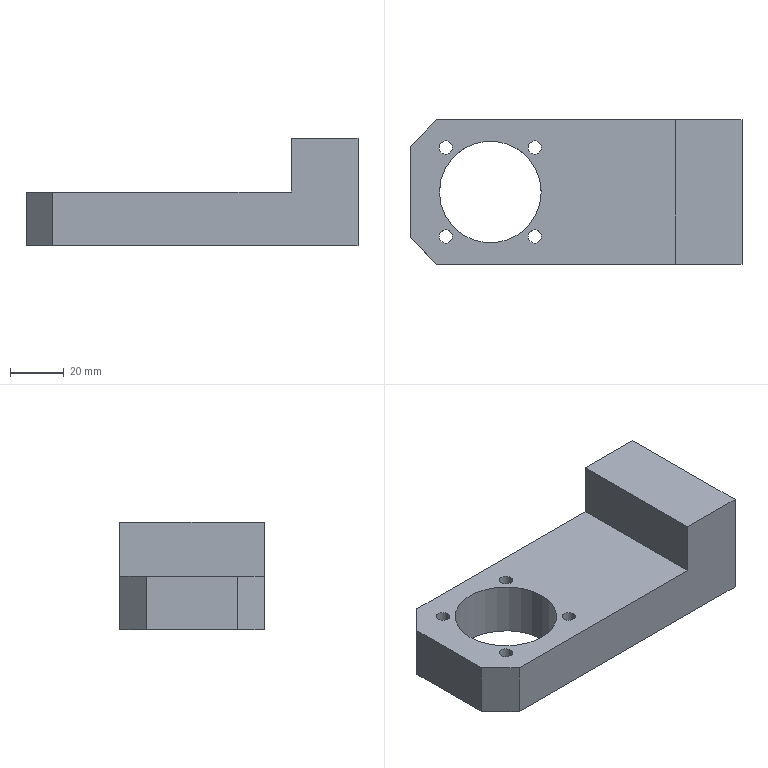Part | SolidWorks | features HoleWzd 2, ICE 2, Chamfer 1, CirPattern 1, Extrusion 1 | 1 solid | 44 faces | box 124 x 54 x 40 mm | volume 132841 mm3 | cylinder 22 | cone 12 | plane 10 | commonest cylinder face diameters 5 x20 38 x2
STEP:
#1=CARTESIAN_POINT('',(109.,47.,37.5));
#2=VERTEX_POINT('',#1);
#3=CARTESIAN_POINT('',(109.,47.,32.5));
#4=VERTEX_POINT('',#3);
#5=CARTESIAN_POINT('',(109.,47.,35.));
#6=DIRECTION('',(1.,0.,0.));
#7=DIRECTION('',(0.,0.,-1.));
#8=AXIS2_PLACEMENT_3D('',#5,#6,#7);
#9=CIRCLE('',#8,2.5);
#10=EDGE_CURVE('',#2,#4,#9,.T.);
#11=ORIENTED_EDGE('',*,*,#10,.F.);
#12=CARTESIAN_POINT('',(124.,47.,37.5));
#13=VERTEX_POINT('',#12);
#14=CARTESIAN_POINT('',(124.,47.,37.5));
#15=DIRECTION('',(1.,0.,0.));
#16=VECTOR('',#15,1000.);
#17=LINE('',#14,#16);
#18=EDGE_CURVE('',#2,#13,#17,.T.);
#19=ORIENTED_EDGE('',*,*,#18,.T.);
#20=CARTESIAN_POINT('',(124.,47.,32.5));
#21=VERTEX_POINT('',#20);
#22=CARTESIAN_POINT('',(124.,47.,35.));
#23=DIRECTION('',(1.,0.,0.));
#24=DIRECTION('',(0.,0.,-1.));
#25=AXIS2_PLACEMENT_3D('',#22,#23,#24);
#26=CIRCLE('',#25,2.5);
#27=EDGE_CURVE('',#13,#21,#26,.T.);
#28=ORIENTED_EDGE('',*,*,#27,.T.);
#29=CARTESIAN_POINT('',(124.,47.,32.5));
#30=DIRECTION('',(1.,0.,0.));
#31=VECTOR('',#30,1000.);
#32=LINE('',#29,#31);
#33=EDGE_CURVE('',#4,#21,#32,.T.);
#34=ORIENTED_EDGE('',*,*,#33,.F.);
#35=EDGE_LOOP('',(#11,#19,#28,#34));
#36=FACE_OUTER_BOUND('',#35,.T.);
#37=CARTESIAN_POINT('',(124.,47.,35.));
#38=DIRECTION('',(1.,0.,0.));
#39=DIRECTION('',(0.,0.,-1.));
#40=AXIS2_PLACEMENT_3D('',#37,#38,#39);
#41=CYLINDRICAL_SURFACE('',#40,2.5);
#42=ADVANCED_FACE('',(#36),#41,.F.);
#43=CARTESIAN_POINT('',(107.498,47.,35.));
#44=VERTEX_POINT('',#43);
#45=CARTESIAN_POINT('',(109.,47.,32.5));
#46=DIRECTION('',(0.515,0.,-0.8572));
#47=VECTOR('',#46,1000.);
#48=LINE('',#45,#47);
#49=EDGE_CURVE('',#44,#4,#48,.T.);
#50=ORIENTED_EDGE('',*,*,#49,.F.);
#51=CARTESIAN_POINT('',(109.,47.,37.5));
#52=DIRECTION('',(0.515,0.,0.8572));
#53=VECTOR('',#52,1000.);
#54=LINE('',#51,#53);
#55=EDGE_CURVE('',#44,#2,#54,.T.);
#56=ORIENTED_EDGE('',*,*,#55,.T.);
#57=ORIENTED_EDGE('',*,*,#10,.T.);
#58=EDGE_LOOP('',(#50,#56,#57));
#59=FACE_OUTER_BOUND('',#58,.T.);
#60=CARTESIAN_POINT('',(109.,47.,35.));
#61=DIRECTION('',(1.,0.,0.));
#62=DIRECTION('',(0.,0.,-1.));
#63=AXIS2_PLACEMENT_3D('',#60,#61,#62);
#64=CONICAL_SURFACE('',#63,2.5,1.03);
#65=ADVANCED_FACE('',(#59),#64,.F.);
#66=CARTESIAN_POINT('',(109.,47.,7.5));
#67=VERTEX_POINT('',#66);
#68=CARTESIAN_POINT('',(109.,47.,2.5));
#69=VERTEX_POINT('',#68);
#70=CARTESIAN_POINT('',(109.,47.,5.));
#71=DIRECTION('',(1.,0.,0.));
#72=DIRECTION('',(0.,0.,-1.));
#73=AXIS2_PLACEMENT_3D('',#70,#71,#72);
#74=CIRCLE('',#73,2.5);
#75=EDGE_CURVE('',#67,#69,#74,.T.);
#76=ORIENTED_EDGE('',*,*,#75,.F.);
#77=CARTESIAN_POINT('',(124.,47.,7.5));
#78=VERTEX_POINT('',#77);
#79=CARTESIAN_POINT('',(124.,47.,7.5));
#80=DIRECTION('',(1.,0.,0.));
#81=VECTOR('',#80,1000.);
#82=LINE('',#79,#81);
#83=EDGE_CURVE('',#67,#78,#82,.T.);
#84=ORIENTED_EDGE('',*,*,#83,.T.);
#85=CARTESIAN_POINT('',(124.,47.,2.5));
#86=VERTEX_POINT('',#85);
#87=CARTESIAN_POINT('',(124.,47.,5.));
#88=DIRECTION('',(1.,0.,0.));
#89=DIRECTION('',(0.,0.,-1.));
#90=AXIS2_PLACEMENT_3D('',#87,#88,#89);
#91=CIRCLE('',#90,2.5);
#92=EDGE_CURVE('',#78,#86,#91,.T.);
#93=ORIENTED_EDGE('',*,*,#92,.T.);
#94=CARTESIAN_POINT('',(124.,47.,2.5));
#95=DIRECTION('',(1.,0.,0.));
#96=VECTOR('',#95,1000.);
#97=LINE('',#94,#96);
#98=EDGE_CURVE('',#69,#86,#97,.T.);
#99=ORIENTED_EDGE('',*,*,#98,.F.);
#100=EDGE_LOOP('',(#76,#84,#93,#99));
#101=FACE_OUTER_BOUND('',#100,.T.);
#102=CARTESIAN_POINT('',(124.,47.,5.));
#103=DIRECTION('',(1.,0.,0.));
#104=DIRECTION('',(0.,0.,-1.));
#105=AXIS2_PLACEMENT_3D('',#102,#103,#104);
#106=CYLINDRICAL_SURFACE('',#105,2.5);
#107=ADVANCED_FACE('',(#101),#106,.F.);
#108=CARTESIAN_POINT('',(107.498,47.,5.));
#109=VERTEX_POINT('',#108);
#110=CARTESIAN_POINT('',(109.,47.,2.5));
#111=DIRECTION('',(0.515,0.,-0.8572));
#112=VECTOR('',#111,1000.);
#113=LINE('',#110,#112);
#114=EDGE_CURVE('',#109,#69,#113,.T.);
#115=ORIENTED_EDGE('',*,*,#114,.F.);
#116=CARTESIAN_POINT('',(109.,47.,7.5));
#117=DIRECTION('',(0.515,0.,0.8572));
#118=VECTOR('',#117,1000.);
#119=LINE('',#116,#118);
#120=EDGE_CURVE('',#109,#67,#119,.T.);
#121=ORIENTED_EDGE('',*,*,#120,.T.);
#122=ORIENTED_EDGE('',*,*,#75,.T.);
#123=EDGE_LOOP('',(#115,#121,#122));
#124=FACE_OUTER_BOUND('',#123,.T.);
#125=CARTESIAN_POINT('',(109.,47.,5.));
#126=DIRECTION('',(1.,0.,0.));
#127=DIRECTION('',(0.,0.,-1.));
#128=AXIS2_PLACEMENT_3D('',#125,#126,#127);
#129=CONICAL_SURFACE('',#128,2.5,1.03);
#130=ADVANCED_FACE('',(#124),#129,.F.);
#131=CARTESIAN_POINT('',(109.,7.,37.5));
#132=VERTEX_POINT('',#131);
#133=CARTESIAN_POINT('',(109.,7.,32.5));
#134=VERTEX_POINT('',#133);
#135=CARTESIAN_POINT('',(109.,7.,35.));
#136=DIRECTION('',(1.,0.,0.));
#137=DIRECTION('',(0.,0.,-1.));
#138=AXIS2_PLACEMENT_3D('',#135,#136,#137);
#139=CIRCLE('',#138,2.5);
#140=EDGE_CURVE('',#132,#134,#139,.T.);
#141=ORIENTED_EDGE('',*,*,#140,.F.);
#142=CARTESIAN_POINT('',(124.,7.,37.5));
#143=VERTEX_POINT('',#142);
#144=CARTESIAN_POINT('',(124.,7.,37.5));
#145=DIRECTION('',(1.,0.,0.));
#146=VECTOR('',#145,1000.);
#147=LINE('',#144,#146);
#148=EDGE_CURVE('',#132,#143,#147,.T.);
#149=ORIENTED_EDGE('',*,*,#148,.T.);
#150=CARTESIAN_POINT('',(124.,7.,32.5));
#151=VERTEX_POINT('',#150);
#152=CARTESIAN_POINT('',(124.,7.,35.));
#153=DIRECTION('',(1.,0.,0.));
#154=DIRECTION('',(0.,0.,-1.));
#155=AXIS2_PLACEMENT_3D('',#152,#153,#154);
#156=CIRCLE('',#155,2.5);
#157=EDGE_CURVE('',#143,#151,#156,.T.);
#158=ORIENTED_EDGE('',*,*,#157,.T.);
#159=CARTESIAN_POINT('',(124.,7.,32.5));
#160=DIRECTION('',(1.,0.,0.));
#161=VECTOR('',#160,1000.);
#162=LINE('',#159,#161);
#163=EDGE_CURVE('',#134,#151,#162,.T.);
#164=ORIENTED_EDGE('',*,*,#163,.F.);
#165=EDGE_LOOP('',(#141,#149,#158,#164));
#166=FACE_OUTER_BOUND('',#165,.T.);
#167=CARTESIAN_POINT('',(124.,7.,35.));
#168=DIRECTION('',(1.,0.,0.));
#169=DIRECTION('',(0.,0.,-1.));
#170=AXIS2_PLACEMENT_3D('',#167,#168,#169);
#171=CYLINDRICAL_SURFACE('',#170,2.5);
#172=ADVANCED_FACE('',(#166),#171,.F.);
#173=CARTESIAN_POINT('',(107.498,7.,35.));
#174=VERTEX_POINT('',#173);
#175=CARTESIAN_POINT('',(109.,7.,32.5));
#176=DIRECTION('',(0.515,0.,-0.8572));
#177=VECTOR('',#176,1000.);
#178=LINE('',#175,#177);
#179=EDGE_CURVE('',#174,#134,#178,.T.);
#180=ORIENTED_EDGE('',*,*,#179,.F.);
#181=CARTESIAN_POINT('',(109.,7.,37.5));
#182=DIRECTION('',(0.515,0.,0.8572));
#183=VECTOR('',#182,1000.);
#184=LINE('',#181,#183);
#185=EDGE_CURVE('',#174,#132,#184,.T.);
#186=ORIENTED_EDGE('',*,*,#185,.T.);
#187=ORIENTED_EDGE('',*,*,#140,.T.);
#188=EDGE_LOOP('',(#180,#186,#187));
#189=FACE_OUTER_BOUND('',#188,.T.);
#190=CARTESIAN_POINT('',(109.,7.,35.));
#191=DIRECTION('',(1.,0.,0.));
#192=DIRECTION('',(0.,0.,-1.));
#193=AXIS2_PLACEMENT_3D('',#190,#191,#192);
#194=CONICAL_SURFACE('',#193,2.5,1.03);
#195=ADVANCED_FACE('',(#189),#194,.F.);
#196=CARTESIAN_POINT('',(109.,7.,7.5));
#197=VERTEX_POINT('',#196);
#198=CARTESIAN_POINT('',(109.,7.,2.5));
#199=VERTEX_POINT('',#198);
#200=CARTESIAN_POINT('',(109.,7.,5.));
#201=DIRECTION('',(1.,0.,0.));
#202=DIRECTION('',(0.,0.,-1.));
#203=AXIS2_PLACEMENT_3D('',#200,#201,#202);
#204=CIRCLE('',#203,2.5);
#205=EDGE_CURVE('',#197,#199,#204,.T.);
#206=ORIENTED_EDGE('',*,*,#205,.F.);
#207=CARTESIAN_POINT('',(124.,7.,7.5));
#208=VERTEX_POINT('',#207);
#209=CARTESIAN_POINT('',(124.,7.,7.5));
#210=DIRECTION('',(1.,0.,0.));
#211=VECTOR('',#210,1000.);
#212=LINE('',#209,#211);
#213=EDGE_CURVE('',#197,#208,#212,.T.);
#214=ORIENTED_EDGE('',*,*,#213,.T.);
#215=CARTESIAN_POINT('',(124.,7.,2.5));
#216=VERTEX_POINT('',#215);
#217=CARTESIAN_POINT('',(124.,7.,5.));
#218=DIRECTION('',(1.,0.,0.));
#219=DIRECTION('',(0.,0.,-1.));
#220=AXIS2_PLACEMENT_3D('',#217,#218,#219);
#221=CIRCLE('',#220,2.5);
#222=EDGE_CURVE('',#208,#216,#221,.T.);
#223=ORIENTED_EDGE('',*,*,#222,.T.);
#224=CARTESIAN_POINT('',(124.,7.,2.5));
#225=DIRECTION('',(1.,0.,0.));
#226=VECTOR('',#225,1000.);
#227=LINE('',#224,#226);
#228=EDGE_CURVE('',#199,#216,#227,.T.);
#229=ORIENTED_EDGE('',*,*,#228,.F.);
#230=EDGE_LOOP('',(#206,#214,#223,#229));
#231=FACE_OUTER_BOUND('',#230,.T.);
#232=CARTESIAN_POINT('',(124.,7.,5.));
#233=DIRECTION('',(1.,0.,0.));
#234=DIRECTION('',(0.,0.,-1.));
#235=AXIS2_PLACEMENT_3D('',#232,#233,#234);
#236=CYLINDRICAL_SURFACE('',#235,2.5);
#237=ADVANCED_FACE('',(#231),#236,.F.);
#238=CARTESIAN_POINT('',(107.498,7.,5.));
#239=VERTEX_POINT('',#238);
#240=CARTESIAN_POINT('',(109.,7.,2.5));
#241=DIRECTION('',(0.515,0.,-0.8572));
#242=VECTOR('',#241,1000.);
#243=LINE('',#240,#242);
#244=EDGE_CURVE('',#239,#199,#243,.T.);
#245=ORIENTED_EDGE('',*,*,#244,.F.);
#246=CARTESIAN_POINT('',(109.,7.,7.5));
#247=DIRECTION('',(0.515,0.,0.8572));
#248=VECTOR('',#247,1000.);
#249=LINE('',#246,#248);
#250=EDGE_CURVE('',#239,#197,#249,.T.);
#251=ORIENTED_EDGE('',*,*,#250,.T.);
#252=ORIENTED_EDGE('',*,*,#205,.T.);
#253=EDGE_LOOP('',(#245,#251,#252));
#254=FACE_OUTER_BOUND('',#253,.T.);
#255=CARTESIAN_POINT('',(109.,7.,5.));
#256=DIRECTION('',(1.,0.,0.));
#257=DIRECTION('',(0.,0.,-1.));
#258=AXIS2_PLACEMENT_3D('',#255,#256,#257);
#259=CONICAL_SURFACE('',#258,2.5,1.03);
#260=ADVANCED_FACE('',(#254),#259,.F.);
#261=CARTESIAN_POINT('',(109.,27.,37.5));
#262=VERTEX_POINT('',#261);
#263=CARTESIAN_POINT('',(109.,27.,32.5));
#264=VERTEX_POINT('',#263);
#265=CARTESIAN_POINT('',(109.,27.,35.));
#266=DIRECTION('',(1.,0.,0.));
#267=DIRECTION('',(0.,0.,-1.));
#268=AXIS2_PLACEMENT_3D('',#265,#266,#267);
#269=CIRCLE('',#268,2.5);
#270=EDGE_CURVE('',#262,#264,#269,.T.);
#271=ORIENTED_EDGE('',*,*,#270,.F.);
#272=CARTESIAN_POINT('',(124.,27.,37.5));
#273=VERTEX_POINT('',#272);
#274=CARTESIAN_POINT('',(124.,27.,37.5));
#275=DIRECTION('',(1.,0.,0.));
#276=VECTOR('',#275,1000.);
#277=LINE('',#274,#276);
#278=EDGE_CURVE('',#262,#273,#277,.T.);
#279=ORIENTED_EDGE('',*,*,#278,.T.);
#280=CARTESIAN_POINT('',(124.,27.,32.5));
#281=VERTEX_POINT('',#280);
#282=CARTESIAN_POINT('',(124.,27.,35.));
#283=DIRECTION('',(1.,0.,0.));
#284=DIRECTION('',(0.,0.,-1.));
#285=AXIS2_PLACEMENT_3D('',#282,#283,#284);
#286=CIRCLE('',#285,2.5);
#287=EDGE_CURVE('',#273,#281,#286,.T.);
#288=ORIENTED_EDGE('',*,*,#287,.T.);
#289=CARTESIAN_POINT('',(124.,27.,32.5));
#290=DIRECTION('',(1.,0.,0.));
#291=VECTOR('',#290,1000.);
#292=LINE('',#289,#291);
#293=EDGE_CURVE('',#264,#281,#292,.T.);
#294=ORIENTED_EDGE('',*,*,#293,.F.);
#295=EDGE_LOOP('',(#271,#279,#288,#294));
#296=FACE_OUTER_BOUND('',#295,.T.);
#297=CARTESIAN_POINT('',(124.,27.,35.));
#298=DIRECTION('',(1.,0.,0.));
#299=DIRECTION('',(0.,0.,-1.));
#300=AXIS2_PLACEMENT_3D('',#297,#298,#299);
#301=CYLINDRICAL_SURFACE('',#300,2.5);
#302=ADVANCED_FACE('',(#296),#301,.F.);
#303=CARTESIAN_POINT('',(107.498,27.,35.));
#304=VERTEX_POINT('',#303);
#305=CARTESIAN_POINT('',(109.,27.,32.5));
#306=DIRECTION('',(0.515,0.,-0.8572));
#307=VECTOR('',#306,1000.);
#308=LINE('',#305,#307);
#309=EDGE_CURVE('',#304,#264,#308,.T.);
#310=ORIENTED_EDGE('',*,*,#309,.F.);
#311=CARTESIAN_POINT('',(109.,27.,37.5));
#312=DIRECTION('',(0.515,0.,0.8572));
#313=VECTOR('',#312,1000.);
#314=LINE('',#311,#313);
#315=EDGE_CURVE('',#304,#262,#314,.T.);
#316=ORIENTED_EDGE('',*,*,#315,.T.);
#317=ORIENTED_EDGE('',*,*,#270,.T.);
#318=EDGE_LOOP('',(#310,#316,#317));
#319=FACE_OUTER_BOUND('',#318,.T.);
#320=CARTESIAN_POINT('',(109.,27.,35.));
#321=DIRECTION('',(1.,0.,0.));
#322=DIRECTION('',(0.,0.,-1.));
#323=AXIS2_PLACEMENT_3D('',#320,#321,#322);
#324=CONICAL_SURFACE('',#323,2.5,1.03);
#325=ADVANCED_FACE('',(#319),#324,.F.);
#326=CARTESIAN_POINT('',(109.,27.,7.5));
#327=VERTEX_POINT('',#326);
#328=CARTESIAN_POINT('',(109.,27.,2.5));
#329=VERTEX_POINT('',#328);
#330=CARTESIAN_POINT('',(109.,27.,5.));
#331=DIRECTION('',(1.,0.,0.));
#332=DIRECTION('',(0.,0.,-1.));
#333=AXIS2_PLACEMENT_3D('',#330,#331,#332);
#334=CIRCLE('',#333,2.5);
#335=EDGE_CURVE('',#327,#329,#334,.T.);
#336=ORIENTED_EDGE('',*,*,#335,.F.);
#337=CARTESIAN_POINT('',(124.,27.,7.5));
#338=VERTEX_POINT('',#337);
#339=CARTESIAN_POINT('',(124.,27.,7.5));
#340=DIRECTION('',(1.,0.,0.));
#341=VECTOR('',#340,1000.);
#342=LINE('',#339,#341);
#343=EDGE_CURVE('',#327,#338,#342,.T.);
#344=ORIENTED_EDGE('',*,*,#343,.T.);
#345=CARTESIAN_POINT('',(124.,27.,2.5));
#346=VERTEX_POINT('',#345);
#347=CARTESIAN_POINT('',(124.,27.,5.));
#348=DIRECTION('',(1.,0.,0.));
#349=DIRECTION('',(0.,0.,-1.));
#350=AXIS2_PLACEMENT_3D('',#347,#348,#349);
#351=CIRCLE('',#350,2.5);
#352=EDGE_CURVE('',#338,#346,#351,.T.);
#353=ORIENTED_EDGE('',*,*,#352,.T.);
#354=CARTESIAN_POINT('',(124.,27.,2.5));
#355=DIRECTION('',(1.,0.,0.));
#356=VECTOR('',#355,1000.);
#357=LINE('',#354,#356);
#358=EDGE_CURVE('',#329,#346,#357,.T.);
#359=ORIENTED_EDGE('',*,*,#358,.F.);
#360=EDGE_LOOP('',(#336,#344,#353,#359));
#361=FACE_OUTER_BOUND('',#360,.T.);
#362=CARTESIAN_POINT('',(124.,27.,5.));
#363=DIRECTION('',(1.,0.,0.));
#364=DIRECTION('',(0.,0.,-1.));
#365=AXIS2_PLACEMENT_3D('',#362,#363,#364);
#366=CYLINDRICAL_SURFACE('',#365,2.5);
#367=ADVANCED_FACE('',(#361),#366,.F.);
#368=CARTESIAN_POINT('',(107.498,27.,5.));
#369=VERTEX_POINT('',#368);
#370=CARTESIAN_POINT('',(109.,27.,2.5));
#371=DIRECTION('',(0.515,0.,-0.8572));
#372=VECTOR('',#371,1000.);
#373=LINE('',#370,#372);
#374=EDGE_CURVE('',#369,#329,#373,.T.);
#375=ORIENTED_EDGE('',*,*,#374,.F.);
#376=CARTESIAN_POINT('',(109.,27.,7.5));
#377=DIRECTION('',(0.515,0.,0.8572));
#378=VECTOR('',#377,1000.);
#379=LINE('',#376,#378);
#380=EDGE_CURVE('',#369,#327,#379,.T.);
#381=ORIENTED_EDGE('',*,*,#380,.T.);
#382=ORIENTED_EDGE('',*,*,#335,.T.);
#383=EDGE_LOOP('',(#375,#381,#382));
#384=FACE_OUTER_BOUND('',#383,.T.);
#385=CARTESIAN_POINT('',(109.,27.,5.));
#386=DIRECTION('',(1.,0.,0.));
#387=DIRECTION('',(0.,0.,-1.));
#388=AXIS2_PLACEMENT_3D('',#385,#386,#387);
#389=CONICAL_SURFACE('',#388,2.5,1.03);
#390=ADVANCED_FACE('',(#384),#389,.F.);
#391=CARTESIAN_POINT('',(44.117,10.383,0.));
#392=VERTEX_POINT('',#391);
#393=CARTESIAN_POINT('',(49.117,10.383,0.));
#394=VERTEX_POINT('',#393);
#395=CARTESIAN_POINT('',(46.617,10.383,0.));
#396=DIRECTION('',(0.,0.,1.));
#397=DIRECTION('',(1.,0.,0.));
#398=AXIS2_PLACEMENT_3D('',#395,#396,#397);
#399=CIRCLE('',#398,2.5);
#400=EDGE_CURVE('',#392,#394,#399,.T.);
#401=ORIENTED_EDGE('',*,*,#400,.F.);
#402=CARTESIAN_POINT('',(44.117,10.383,20.));
#403=VERTEX_POINT('',#402);
#404=CARTESIAN_POINT('',(44.117,10.383,20.));
#405=DIRECTION('',(0.,0.,1.));
#406=VECTOR('',#405,1000.);
#407=LINE('',#404,#406);
#408=EDGE_CURVE('',#392,#403,#407,.T.);
#409=ORIENTED_EDGE('',*,*,#408,.T.);
#410=CARTESIAN_POINT('',(49.117,10.383,20.));
#411=VERTEX_POINT('',#410);
#412=CARTESIAN_POINT('',(46.617,10.383,20.));
#413=DIRECTION('',(0.,0.,1.));
#414=DIRECTION('',(1.,0.,0.));
#415=AXIS2_PLACEMENT_3D('',#412,#413,#414);
#416=CIRCLE('',#415,2.5);
#417=EDGE_CURVE('',#403,#411,#416,.T.);
#418=ORIENTED_EDGE('',*,*,#417,.T.);
#419=CARTESIAN_POINT('',(49.117,10.383,20.));
#420=DIRECTION('',(0.,0.,1.));
#421=VECTOR('',#420,1000.);
#422=LINE('',#419,#421);
#423=EDGE_CURVE('',#394,#411,#422,.T.);
#424=ORIENTED_EDGE('',*,*,#423,.F.);
#425=EDGE_LOOP('',(#401,#409,#418,#424));
#426=FACE_OUTER_BOUND('',#425,.T.);
#427=CARTESIAN_POINT('',(46.617,10.383,20.));
#428=DIRECTION('',(0.,0.,1.));
#429=DIRECTION('',(1.,0.,0.));
#430=AXIS2_PLACEMENT_3D('',#427,#428,#429);
#431=CYLINDRICAL_SURFACE('',#430,2.5);
#432=ADVANCED_FACE('',(#426),#431,.F.);
#433=CARTESIAN_POINT('',(10.883,10.383,0.));
#434=VERTEX_POINT('',#433);
#435=CARTESIAN_POINT('',(15.883,10.383,0.));
#436=VERTEX_POINT('',#435);
#437=CARTESIAN_POINT('',(13.383,10.383,0.));
#438=DIRECTION('',(0.,0.,1.));
#439=DIRECTION('',(1.,0.,0.));
#440=AXIS2_PLACEMENT_3D('',#437,#438,#439);
#441=CIRCLE('',#440,2.5);
#442=EDGE_CURVE('',#434,#436,#441,.T.);
#443=ORIENTED_EDGE('',*,*,#442,.F.);
#444=CARTESIAN_POINT('',(10.883,10.383,20.));
#445=VERTEX_POINT('',#444);
#446=CARTESIAN_POINT('',(10.883,10.383,20.));
#447=DIRECTION('',(0.,0.,1.));
#448=VECTOR('',#447,1000.);
#449=LINE('',#446,#448);
#450=EDGE_CURVE('',#434,#445,#449,.T.);
#451=ORIENTED_EDGE('',*,*,#450,.T.);
#452=CARTESIAN_POINT('',(15.883,10.383,20.));
#453=VERTEX_POINT('',#452);
#454=CARTESIAN_POINT('',(13.383,10.383,20.));
#455=DIRECTION('',(0.,0.,1.));
#456=DIRECTION('',(1.,0.,0.));
#457=AXIS2_PLACEMENT_3D('',#454,#455,#456);
#458=CIRCLE('',#457,2.5);
#459=EDGE_CURVE('',#445,#453,#458,.T.);
#460=ORIENTED_EDGE('',*,*,#459,.T.);
#461=CARTESIAN_POINT('',(15.883,10.383,20.));
#462=DIRECTION('',(0.,0.,1.));
#463=VECTOR('',#462,1000.);
#464=LINE('',#461,#463);
#465=EDGE_CURVE('',#436,#453,#464,.T.);
#466=ORIENTED_EDGE('',*,*,#465,.F.);
#467=EDGE_LOOP('',(#443,#451,#460,#466));
#468=FACE_OUTER_BOUND('',#467,.T.);
#469=CARTESIAN_POINT('',(13.383,10.383,20.));
#470=DIRECTION('',(0.,0.,1.));
#471=DIRECTION('',(1.,0.,0.));
#472=AXIS2_PLACEMENT_3D('',#469,#470,#471);
#473=CYLINDRICAL_SURFACE('',#472,2.5);
#474=ADVANCED_FACE('',(#468),#473,.F.);
#475=CARTESIAN_POINT('',(10.883,43.617,0.));
#476=VERTEX_POINT('',#475);
#477=CARTESIAN_POINT('',(15.883,43.617,0.));
#478=VERTEX_POINT('',#477);
#479=CARTESIAN_POINT('',(13.383,43.617,0.));
#480=DIRECTION('',(0.,0.,1.));
#481=DIRECTION('',(1.,0.,0.));
#482=AXIS2_PLACEMENT_3D('',#479,#480,#481);
#483=CIRCLE('',#482,2.5);
#484=EDGE_CURVE('',#476,#478,#483,.T.);
#485=ORIENTED_EDGE('',*,*,#484,.F.);
#486=CARTESIAN_POINT('',(10.883,43.617,20.));
#487=VERTEX_POINT('',#486);
#488=CARTESIAN_POINT('',(10.883,43.617,20.));
#489=DIRECTION('',(0.,0.,1.));
#490=VECTOR('',#489,1000.);
#491=LINE('',#488,#490);
#492=EDGE_CURVE('',#476,#487,#491,.T.);
#493=ORIENTED_EDGE('',*,*,#492,.T.);
#494=CARTESIAN_POINT('',(15.883,43.617,20.));
#495=VERTEX_POINT('',#494);
#496=CARTESIAN_POINT('',(13.383,43.617,20.));
#497=DIRECTION('',(0.,0.,1.));
#498=DIRECTION('',(1.,0.,0.));
#499=AXIS2_PLACEMENT_3D('',#496,#497,#498);
#500=CIRCLE('',#499,2.5);
#501=EDGE_CURVE('',#487,#495,#500,.T.);
#502=ORIENTED_EDGE('',*,*,#501,.T.);
#503=CARTESIAN_POINT('',(15.883,43.617,20.));
#504=DIRECTION('',(0.,0.,1.));
#505=VECTOR('',#504,1000.);
#506=LINE('',#503,#505);
#507=EDGE_CURVE('',#478,#495,#506,.T.);
#508=ORIENTED_EDGE('',*,*,#507,.F.);
#509=EDGE_LOOP('',(#485,#493,#502,#508));
#510=FACE_OUTER_BOUND('',#509,.T.);
#511=CARTESIAN_POINT('',(13.383,43.617,20.));
#512=DIRECTION('',(0.,0.,1.));
#513=DIRECTION('',(1.,0.,0.));
#514=AXIS2_PLACEMENT_3D('',#511,#512,#513);
#515=CYLINDRICAL_SURFACE('',#514,2.5);
#516=ADVANCED_FACE('',(#510),#515,.F.);
#517=CARTESIAN_POINT('',(44.117,43.617,0.));
#518=VERTEX_POINT('',#517);
#519=CARTESIAN_POINT('',(49.117,43.617,0.));
#520=VERTEX_POINT('',#519);
#521=CARTESIAN_POINT('',(46.617,43.617,0.));
#522=DIRECTION('',(0.,0.,1.));
#523=DIRECTION('',(1.,0.,0.));
#524=AXIS2_PLACEMENT_3D('',#521,#522,#523);
#525=CIRCLE('',#524,2.5);
#526=EDGE_CURVE('',#518,#520,#525,.T.);
#527=ORIENTED_EDGE('',*,*,#526,.F.);
#528=CARTESIAN_POINT('',(44.117,43.617,20.));
#529=VERTEX_POINT('',#528);
#530=CARTESIAN_POINT('',(44.117,43.617,20.));
#531=DIRECTION('',(0.,0.,1.));
#532=VECTOR('',#531,1000.);
#533=LINE('',#530,#532);
#534=EDGE_CURVE('',#518,#529,#533,.T.);
#535=ORIENTED_EDGE('',*,*,#534,.T.);
#536=CARTESIAN_POINT('',(49.117,43.617,20.));
#537=VERTEX_POINT('',#536);
#538=CARTESIAN_POINT('',(46.617,43.617,20.));
#539=DIRECTION('',(0.,0.,1.));
#540=DIRECTION('',(1.,0.,0.));
#541=AXIS2_PLACEMENT_3D('',#538,#539,#540);
#542=CIRCLE('',#541,2.5);
#543=EDGE_CURVE('',#529,#537,#542,.T.);
#544=ORIENTED_EDGE('',*,*,#543,.T.);
#545=CARTESIAN_POINT('',(49.117,43.617,20.));
#546=DIRECTION('',(0.,0.,1.));
#547=VECTOR('',#546,1000.);
#548=LINE('',#545,#547);
#549=EDGE_CURVE('',#520,#537,#548,.T.);
#550=ORIENTED_EDGE('',*,*,#549,.F.);
#551=EDGE_LOOP('',(#527,#535,#544,#550));
#552=FACE_OUTER_BOUND('',#551,.T.);
#553=CARTESIAN_POINT('',(46.617,43.617,20.));
#554=DIRECTION('',(0.,0.,1.));
#555=DIRECTION('',(1.,0.,0.));
#556=AXIS2_PLACEMENT_3D('',#553,#554,#555);
#557=CYLINDRICAL_SURFACE('',#556,2.5);
#558=ADVANCED_FACE('',(#552),#557,.F.);
#559=CARTESIAN_POINT('',(11.,27.,0.));
#560=VERTEX_POINT('',#559);
#561=CARTESIAN_POINT('',(49.,27.,0.));
#562=VERTEX_POINT('',#561);
#563=CARTESIAN_POINT('',(30.,27.,0.));
#564=DIRECTION('',(0.,0.,1.));
#565=DIRECTION('',(1.,0.,0.));
#566=AXIS2_PLACEMENT_3D('',#563,#564,#565);
#567=CIRCLE('',#566,19.);
#568=EDGE_CURVE('',#560,#562,#567,.T.);
#569=ORIENTED_EDGE('',*,*,#568,.F.);
#570=CARTESIAN_POINT('',(11.,27.,20.));
#571=VERTEX_POINT('',#570);
#572=CARTESIAN_POINT('',(11.,27.,0.));
#573=DIRECTION('',(0.,0.,1.));
#574=VECTOR('',#573,1000.);
#575=LINE('',#572,#574);
#576=EDGE_CURVE('',#560,#571,#575,.T.);
#577=ORIENTED_EDGE('',*,*,#576,.T.);
#578=CARTESIAN_POINT('',(49.,27.,20.));
#579=VERTEX_POINT('',#578);
#580=CARTESIAN_POINT('',(30.,27.,20.));
#581=DIRECTION('',(0.,0.,1.));
#582=DIRECTION('',(1.,0.,0.));
#583=AXIS2_PLACEMENT_3D('',#580,#581,#582);
#584=CIRCLE('',#583,19.);
#585=EDGE_CURVE('',#571,#579,#584,.T.);
#586=ORIENTED_EDGE('',*,*,#585,.T.);
#587=CARTESIAN_POINT('',(49.,27.,0.));
#588=DIRECTION('',(0.,0.,1.));
#589=VECTOR('',#588,1000.);
#590=LINE('',#587,#589);
#591=EDGE_CURVE('',#562,#579,#590,.T.);
#592=ORIENTED_EDGE('',*,*,#591,.F.);
#593=EDGE_LOOP('',(#569,#577,#586,#592));
#594=FACE_OUTER_BOUND('',#593,.T.);
#595=CARTESIAN_POINT('',(30.,27.,0.));
#596=DIRECTION('',(0.,0.,1.));
#597=DIRECTION('',(1.,0.,0.));
#598=AXIS2_PLACEMENT_3D('',#595,#596,#597);
#599=CYLINDRICAL_SURFACE('',#598,19.);
#600=ADVANCED_FACE('',(#594),#599,.F.);
#601=CARTESIAN_POINT('',(30.,27.,20.));
#602=DIRECTION('',(0.,0.,1.));
#603=DIRECTION('',(1.,0.,0.));
#604=AXIS2_PLACEMENT_3D('',#601,#602,#603);
#605=CIRCLE('',#604,19.);
#606=EDGE_CURVE('',#579,#571,#605,.T.);
#607=ORIENTED_EDGE('',*,*,#606,.F.);
#608=ORIENTED_EDGE('',*,*,#585,.F.);
#609=EDGE_LOOP('',(#607,#608));
#610=FACE_BOUND('',#609,.T.);
#611=CARTESIAN_POINT('',(46.617,43.617,20.));
#612=DIRECTION('',(0.,0.,1.));
#613=DIRECTION('',(1.,0.,0.));
#614=AXIS2_PLACEMENT_3D('',#611,#612,#613);
#615=CIRCLE('',#614,2.5);
#616=EDGE_CURVE('',#537,#529,#615,.T.);
#617=ORIENTED_EDGE('',*,*,#616,.F.);
#618=ORIENTED_EDGE('',*,*,#543,.F.);
#619=EDGE_LOOP('',(#617,#618));
#620=FACE_BOUND('',#619,.T.);
#621=CARTESIAN_POINT('',(13.383,43.617,20.));
#622=DIRECTION('',(0.,0.,1.));
#623=DIRECTION('',(1.,0.,0.));
#624=AXIS2_PLACEMENT_3D('',#621,#622,#623);
#625=CIRCLE('',#624,2.5);
#626=EDGE_CURVE('',#495,#487,#625,.T.);
#627=ORIENTED_EDGE('',*,*,#626,.F.);
#628=ORIENTED_EDGE('',*,*,#501,.F.);
#629=EDGE_LOOP('',(#627,#628));
#630=FACE_BOUND('',#629,.T.);
#631=CARTESIAN_POINT('',(13.383,10.383,20.));
#632=DIRECTION('',(0.,0.,1.));
#633=DIRECTION('',(1.,0.,0.));
#634=AXIS2_PLACEMENT_3D('',#631,#632,#633);
#635=CIRCLE('',#634,2.5);
#636=EDGE_CURVE('',#453,#445,#635,.T.);
#637=ORIENTED_EDGE('',*,*,#636,.F.);
#638=ORIENTED_EDGE('',*,*,#459,.F.);
#639=EDGE_LOOP('',(#637,#638));
#640=FACE_BOUND('',#639,.T.);
#641=CARTESIAN_POINT('',(46.617,10.383,20.));
#642=DIRECTION('',(0.,0.,1.));
#643=DIRECTION('',(1.,0.,0.));
#644=AXIS2_PLACEMENT_3D('',#641,#642,#643);
#645=CIRCLE('',#644,2.5);
#646=EDGE_CURVE('',#411,#403,#645,.T.);
#647=ORIENTED_EDGE('',*,*,#646,.F.);
#648=ORIENTED_EDGE('',*,*,#417,.F.);
#649=EDGE_LOOP('',(#647,#648));
#650=FACE_BOUND('',#649,.T.);
#651=CARTESIAN_POINT('',(99.,54.,20.));
#652=VERTEX_POINT('',#651);
#653=CARTESIAN_POINT('',(99.,0.,20.));
#654=VERTEX_POINT('',#653);
#655=CARTESIAN_POINT('',(99.,0.,20.));
#656=DIRECTION('',(0.,-1.,0.));
#657=VECTOR('',#656,1000.);
#658=LINE('',#655,#657);
#659=EDGE_CURVE('',#652,#654,#658,.T.);
#660=ORIENTED_EDGE('',*,*,#659,.F.);
#661=CARTESIAN_POINT('',(10.,54.,20.));
#662=VERTEX_POINT('',#661);
#663=CARTESIAN_POINT('',(0.,54.,20.));
#664=DIRECTION('',(-1.,0.,0.));
#665=VECTOR('',#664,1000.);
#666=LINE('',#663,#665);
#667=EDGE_CURVE('',#652,#662,#666,.T.);
#668=ORIENTED_EDGE('',*,*,#667,.T.);
#669=CARTESIAN_POINT('',(0.,44.,20.));
#670=VERTEX_POINT('',#669);
#671=CARTESIAN_POINT('',(0.,44.,20.));
#672=DIRECTION('',(-0.7071,-0.7071,0.));
#673=VECTOR('',#672,1000.);
#674=LINE('',#671,#673);
#675=EDGE_CURVE('',#662,#670,#674,.T.);
#676=ORIENTED_EDGE('',*,*,#675,.T.);
#677=CARTESIAN_POINT('',(0.,10.,20.));
#678=VERTEX_POINT('',#677);
#679=CARTESIAN_POINT('',(0.,0.,20.));
#680=DIRECTION('',(0.,-1.,0.));
#681=VECTOR('',#680,1000.);
#682=LINE('',#679,#681);
#683=EDGE_CURVE('',#670,#678,#682,.T.);
#684=ORIENTED_EDGE('',*,*,#683,.T.);
#685=CARTESIAN_POINT('',(10.,0.,20.));
#686=VERTEX_POINT('',#685);
#687=CARTESIAN_POINT('',(10.,0.,20.));
#688=DIRECTION('',(0.7071,-0.7071,0.));
#689=VECTOR('',#688,1000.);
#690=LINE('',#687,#689);
#691=EDGE_CURVE('',#678,#686,#690,.T.);
#692=ORIENTED_EDGE('',*,*,#691,.T.);
#693=CARTESIAN_POINT('',(0.,0.,20.));
#694=DIRECTION('',(1.,0.,0.));
#695=VECTOR('',#694,1000.);
#696=LINE('',#693,#695);
#697=EDGE_CURVE('',#686,#654,#696,.T.);
#698=ORIENTED_EDGE('',*,*,#697,.T.);
#699=EDGE_LOOP('',(#660,#668,#676,#684,#692,#698));
#700=FACE_OUTER_BOUND('',#699,.T.);
#701=CARTESIAN_POINT('',(0.,54.,20.));
#702=DIRECTION('',(0.,0.,-1.));
#703=DIRECTION('',(-1.,0.,0.));
#704=AXIS2_PLACEMENT_3D('',#701,#702,#703);
#705=PLANE('',#704);
#706=ADVANCED_FACE('',(#610,#620,#630,#640,#650,#700),#705,.F.);
#707=CARTESIAN_POINT('',(0.,44.,0.));
#708=VERTEX_POINT('',#707);
#709=CARTESIAN_POINT('',(0.,10.,0.));
#710=VERTEX_POINT('',#709);
#711=CARTESIAN_POINT('',(0.,0.,0.));
#712=DIRECTION('',(0.,-1.,0.));
#713=VECTOR('',#712,1000.);
#714=LINE('',#711,#713);
#715=EDGE_CURVE('',#708,#710,#714,.T.);
#716=ORIENTED_EDGE('',*,*,#715,.F.);
#717=CARTESIAN_POINT('',(10.,54.,0.));
#718=VERTEX_POINT('',#717);
#719=CARTESIAN_POINT('',(5.,49.,0.));
#720=DIRECTION('',(0.7071,0.7071,0.));
#721=VECTOR('',#720,1000.);
#722=LINE('',#719,#721);
#723=EDGE_CURVE('',#708,#718,#722,.T.);
#724=ORIENTED_EDGE('',*,*,#723,.T.);
#725=CARTESIAN_POINT('',(124.,54.,0.));
#726=VERTEX_POINT('',#725);
#727=CARTESIAN_POINT('',(0.,54.,0.));
#728=DIRECTION('',(-1.,0.,0.));
#729=VECTOR('',#728,1000.);
#730=LINE('',#727,#729);
#731=EDGE_CURVE('',#726,#718,#730,.T.);
#732=ORIENTED_EDGE('',*,*,#731,.F.);
#733=CARTESIAN_POINT('',(124.,0.,0.));
#734=VERTEX_POINT('',#733);
#735=CARTESIAN_POINT('',(124.,0.,0.));
#736=DIRECTION('',(0.,1.,0.));
#737=VECTOR('',#736,1000.);
#738=LINE('',#735,#737);
#739=EDGE_CURVE('',#734,#726,#738,.T.);
#740=ORIENTED_EDGE('',*,*,#739,.F.);
#741=CARTESIAN_POINT('',(10.,0.,0.));
#742=VERTEX_POINT('',#741);
#743=CARTESIAN_POINT('',(0.,0.,0.));
#744=DIRECTION('',(1.,0.,0.));
#745=VECTOR('',#744,1000.);
#746=LINE('',#743,#745);
#747=EDGE_CURVE('',#742,#734,#746,.T.);
#748=ORIENTED_EDGE('',*,*,#747,.F.);
#749=CARTESIAN_POINT('',(-22.,32.,0.));
#750=DIRECTION('',(-0.7071,0.7071,0.));
#751=VECTOR('',#750,1000.);
#752=LINE('',#749,#751);
#753=EDGE_CURVE('',#742,#710,#752,.T.);
#754=ORIENTED_EDGE('',*,*,#753,.T.);
#755=EDGE_LOOP('',(#716,#724,#732,#740,#748,#754));
#756=FACE_OUTER_BOUND('',#755,.T.);
#757=CARTESIAN_POINT('',(30.,27.,0.));
#758=DIRECTION('',(0.,0.,1.));
#759=DIRECTION('',(1.,0.,0.));
#760=AXIS2_PLACEMENT_3D('',#757,#758,#759);
#761=CIRCLE('',#760,19.);
#762=EDGE_CURVE('',#562,#560,#761,.T.);
#763=ORIENTED_EDGE('',*,*,#762,.T.);
#764=ORIENTED_EDGE('',*,*,#568,.T.);
#765=EDGE_LOOP('',(#763,#764));
#766=FACE_BOUND('',#765,.T.);
#767=CARTESIAN_POINT('',(46.617,43.617,0.));
#768=DIRECTION('',(0.,0.,1.));
#769=DIRECTION('',(1.,0.,0.));
#770=AXIS2_PLACEMENT_3D('',#767,#768,#769);
#771=CIRCLE('',#770,2.5);
#772=EDGE_CURVE('',#520,#518,#771,.T.);
#773=ORIENTED_EDGE('',*,*,#772,.T.);
#774=ORIENTED_EDGE('',*,*,#526,.T.);
#775=EDGE_LOOP('',(#773,#774));
#776=FACE_BOUND('',#775,.T.);
#777=CARTESIAN_POINT('',(13.383,43.617,0.));
#778=DIRECTION('',(0.,0.,1.));
#779=DIRECTION('',(1.,0.,0.));
#780=AXIS2_PLACEMENT_3D('',#777,#778,#779);
#781=CIRCLE('',#780,2.5);
#782=EDGE_CURVE('',#478,#476,#781,.T.);
#783=ORIENTED_EDGE('',*,*,#782,.T.);
#784=ORIENTED_EDGE('',*,*,#484,.T.);
#785=EDGE_LOOP('',(#783,#784));
#786=FACE_BOUND('',#785,.T.);
#787=CARTESIAN_POINT('',(13.383,10.383,0.));
#788=DIRECTION('',(0.,0.,1.));
#789=DIRECTION('',(1.,0.,0.));
#790=AXIS2_PLACEMENT_3D('',#787,#788,#789);
#791=CIRCLE('',#790,2.5);
#792=EDGE_CURVE('',#436,#434,#791,.T.);
#793=ORIENTED_EDGE('',*,*,#792,.T.);
#794=ORIENTED_EDGE('',*,*,#442,.T.);
#795=EDGE_LOOP('',(#793,#794));
#796=FACE_BOUND('',#795,.T.);
#797=CARTESIAN_POINT('',(46.617,10.383,0.));
#798=DIRECTION('',(0.,0.,1.));
#799=DIRECTION('',(1.,0.,0.));
#800=AXIS2_PLACEMENT_3D('',#797,#798,#799);
#801=CIRCLE('',#800,2.5);
#802=EDGE_CURVE('',#394,#392,#801,.T.);
#803=ORIENTED_EDGE('',*,*,#802,.T.);
#804=ORIENTED_EDGE('',*,*,#400,.T.);
#805=EDGE_LOOP('',(#803,#804));
#806=FACE_BOUND('',#805,.T.);
#807=CARTESIAN_POINT('',(0.,54.,0.));
#808=DIRECTION('',(0.,0.,-1.));
#809=DIRECTION('',(-1.,0.,0.));
#810=AXIS2_PLACEMENT_3D('',#807,#808,#809);
#811=PLANE('',#810);
#812=ADVANCED_FACE('',(#756,#766,#776,#786,#796,#806),#811,.T.);
#813=ORIENTED_EDGE('',*,*,#683,.F.);
#814=CARTESIAN_POINT('',(0.,44.,20.));
#815=DIRECTION('',(0.,0.,-1.));
#816=VECTOR('',#815,1000.);
#817=LINE('',#814,#816);
#818=EDGE_CURVE('',#670,#708,#817,.T.);
#819=ORIENTED_EDGE('',*,*,#818,.T.);
#820=ORIENTED_EDGE('',*,*,#715,.T.);
#821=CARTESIAN_POINT('',(0.,10.,20.));
#822=DIRECTION('',(0.,0.,1.));
#823=VECTOR('',#822,1000.);
#824=LINE('',#821,#823);
#825=EDGE_CURVE('',#710,#678,#824,.T.);
#826=ORIENTED_EDGE('',*,*,#825,.T.);
#827=EDGE_LOOP('',(#813,#819,#820,#826));
#828=FACE_OUTER_BOUND('',#827,.T.);
#829=CARTESIAN_POINT('',(0.,0.,20.));
#830=DIRECTION('',(1.,0.,0.));
#831=DIRECTION('',(0.,0.,-1.));
#832=AXIS2_PLACEMENT_3D('',#829,#830,#831);
#833=PLANE('',#832);
#834=ADVANCED_FACE('',(#828),#833,.F.);
#835=ORIENTED_EDGE('',*,*,#697,.F.);
#836=CARTESIAN_POINT('',(10.,0.,20.));
#837=DIRECTION('',(0.,0.,-1.));
#838=VECTOR('',#837,1000.);
#839=LINE('',#836,#838);
#840=EDGE_CURVE('',#686,#742,#839,.T.);
#841=ORIENTED_EDGE('',*,*,#840,.T.);
#842=ORIENTED_EDGE('',*,*,#747,.T.);
#843=CARTESIAN_POINT('',(124.,0.,40.));
#844=VERTEX_POINT('',#843);
#845=CARTESIAN_POINT('',(124.,0.,20.));
#846=DIRECTION('',(0.,0.,-1.));
#847=VECTOR('',#846,1000.);
#848=LINE('',#845,#847);
#849=EDGE_CURVE('',#844,#734,#848,.T.);
#850=ORIENTED_EDGE('',*,*,#849,.F.);
#851=CARTESIAN_POINT('',(99.,0.,40.));
#852=VERTEX_POINT('',#851);
#853=CARTESIAN_POINT('',(124.,0.,40.));
#854=DIRECTION('',(1.,0.,0.));
#855=VECTOR('',#854,1000.);
#856=LINE('',#853,#855);
#857=EDGE_CURVE('',#852,#844,#856,.T.);
#858=ORIENTED_EDGE('',*,*,#857,.F.);
#859=CARTESIAN_POINT('',(99.,0.,40.));
#860=DIRECTION('',(0.,0.,-1.));
#861=VECTOR('',#860,1000.);
#862=LINE('',#859,#861);
#863=EDGE_CURVE('',#852,#654,#862,.T.);
#864=ORIENTED_EDGE('',*,*,#863,.T.);
#865=EDGE_LOOP('',(#835,#841,#842,#850,#858,#864));
#866=FACE_OUTER_BOUND('',#865,.T.);
#867=CARTESIAN_POINT('',(0.,0.,20.));
#868=DIRECTION('',(0.,1.,0.));
#869=DIRECTION('',(0.,0.,1.));
#870=AXIS2_PLACEMENT_3D('',#867,#868,#869);
#871=PLANE('',#870);
#872=ADVANCED_FACE('',(#866),#871,.F.);
#873=CARTESIAN_POINT('',(124.,47.,35.));
#874=DIRECTION('',(1.,0.,0.));
#875=DIRECTION('',(0.,0.,-1.));
#876=AXIS2_PLACEMENT_3D('',#873,#874,#875);
#877=CIRCLE('',#876,2.5);
#878=EDGE_CURVE('',#21,#13,#877,.T.);
#879=ORIENTED_EDGE('',*,*,#878,.F.);
#880=ORIENTED_EDGE('',*,*,#27,.F.);
#881=EDGE_LOOP('',(#879,#880));
#882=FACE_BOUND('',#881,.T.);
#883=CARTESIAN_POINT('',(124.,47.,5.));
#884=DIRECTION('',(1.,0.,0.));
#885=DIRECTION('',(0.,0.,-1.));
#886=AXIS2_PLACEMENT_3D('',#883,#884,#885);
#887=CIRCLE('',#886,2.5);
#888=EDGE_CURVE('',#86,#78,#887,.T.);
#889=ORIENTED_EDGE('',*,*,#888,.F.);
#890=ORIENTED_EDGE('',*,*,#92,.F.);
#891=EDGE_LOOP('',(#889,#890));
#892=FACE_BOUND('',#891,.T.);
#893=CARTESIAN_POINT('',(124.,7.,35.));
#894=DIRECTION('',(1.,0.,0.));
#895=DIRECTION('',(0.,0.,-1.));
#896=AXIS2_PLACEMENT_3D('',#893,#894,#895);
#897=CIRCLE('',#896,2.5);
#898=EDGE_CURVE('',#151,#143,#897,.T.);
#899=ORIENTED_EDGE('',*,*,#898,.F.);
#900=ORIENTED_EDGE('',*,*,#157,.F.);
#901=EDGE_LOOP('',(#899,#900));
#902=FACE_BOUND('',#901,.T.);
#903=CARTESIAN_POINT('',(124.,7.,5.));
#904=DIRECTION('',(1.,0.,0.));
#905=DIRECTION('',(0.,0.,-1.));
#906=AXIS2_PLACEMENT_3D('',#903,#904,#905);
#907=CIRCLE('',#906,2.5);
#908=EDGE_CURVE('',#216,#208,#907,.T.);
#909=ORIENTED_EDGE('',*,*,#908,.F.);
#910=ORIENTED_EDGE('',*,*,#222,.F.);
#911=EDGE_LOOP('',(#909,#910));
#912=FACE_BOUND('',#911,.T.);
#913=CARTESIAN_POINT('',(124.,27.,35.));
#914=DIRECTION('',(1.,0.,0.));
#915=DIRECTION('',(0.,0.,-1.));
#916=AXIS2_PLACEMENT_3D('',#913,#914,#915);
#917=CIRCLE('',#916,2.5);
#918=EDGE_CURVE('',#281,#273,#917,.T.);
#919=ORIENTED_EDGE('',*,*,#918,.F.);
#920=ORIENTED_EDGE('',*,*,#287,.F.);
#921=EDGE_LOOP('',(#919,#920));
#922=FACE_BOUND('',#921,.T.);
#923=CARTESIAN_POINT('',(124.,27.,5.));
#924=DIRECTION('',(1.,0.,0.));
#925=DIRECTION('',(0.,0.,-1.));
#926=AXIS2_PLACEMENT_3D('',#923,#924,#925);
#927=CIRCLE('',#926,2.5);
#928=EDGE_CURVE('',#346,#338,#927,.T.);
#929=ORIENTED_EDGE('',*,*,#928,.F.);
#930=ORIENTED_EDGE('',*,*,#352,.F.);
#931=EDGE_LOOP('',(#929,#930));
#932=FACE_BOUND('',#931,.T.);
#933=ORIENTED_EDGE('',*,*,#739,.T.);
#934=CARTESIAN_POINT('',(124.,54.,40.));
#935=VERTEX_POINT('',#934);
#936=CARTESIAN_POINT('',(124.,54.,20.));
#937=DIRECTION('',(0.,0.,-1.));
#938=VECTOR('',#937,1000.);
#939=LINE('',#936,#938);
#940=EDGE_CURVE('',#935,#726,#939,.T.);
#941=ORIENTED_EDGE('',*,*,#940,.F.);
#942=CARTESIAN_POINT('',(124.,0.,40.));
#943=DIRECTION('',(0.,1.,0.));
#944=VECTOR('',#943,1000.);
#945=LINE('',#942,#944);
#946=EDGE_CURVE('',#844,#935,#945,.T.);
#947=ORIENTED_EDGE('',*,*,#946,.F.);
#948=ORIENTED_EDGE('',*,*,#849,.T.);
#949=EDGE_LOOP('',(#933,#941,#947,#948));
#950=FACE_OUTER_BOUND('',#949,.T.);
#951=CARTESIAN_POINT('',(124.,0.,20.));
#952=DIRECTION('',(-1.,0.,0.));
#953=DIRECTION('',(0.,0.,1.));
#954=AXIS2_PLACEMENT_3D('',#951,#952,#953);
#955=PLANE('',#954);
#956=ADVANCED_FACE('',(#882,#892,#902,#912,#922,#932,#950),#955,.F.);
#957=ORIENTED_EDGE('',*,*,#731,.T.);
#958=CARTESIAN_POINT('',(10.,54.,20.));
#959=DIRECTION('',(0.,0.,1.));
#960=VECTOR('',#959,1000.);
#961=LINE('',#958,#960);
#962=EDGE_CURVE('',#718,#662,#961,.T.);
#963=ORIENTED_EDGE('',*,*,#962,.T.);
#964=ORIENTED_EDGE('',*,*,#667,.F.);
#965=CARTESIAN_POINT('',(99.,54.,40.));
#966=VERTEX_POINT('',#965);
#967=CARTESIAN_POINT('',(99.,54.,40.));
#968=DIRECTION('',(0.,0.,-1.));
#969=VECTOR('',#968,1000.);
#970=LINE('',#967,#969);
#971=EDGE_CURVE('',#966,#652,#970,.T.);
#972=ORIENTED_EDGE('',*,*,#971,.F.);
#973=CARTESIAN_POINT('',(124.,54.,40.));
#974=DIRECTION('',(-1.,0.,0.));
#975=VECTOR('',#974,1000.);
#976=LINE('',#973,#975);
#977=EDGE_CURVE('',#935,#966,#976,.T.);
#978=ORIENTED_EDGE('',*,*,#977,.F.);
#979=ORIENTED_EDGE('',*,*,#940,.T.);
#980=EDGE_LOOP('',(#957,#963,#964,#972,#978,#979));
#981=FACE_OUTER_BOUND('',#980,.T.);
#982=CARTESIAN_POINT('',(0.,54.,20.));
#983=DIRECTION('',(0.,-1.,0.));
#984=DIRECTION('',(0.,0.,-1.));
#985=AXIS2_PLACEMENT_3D('',#982,#983,#984);
#986=PLANE('',#985);
#987=ADVANCED_FACE('',(#981),#986,.F.);
#988=ORIENTED_EDGE('',*,*,#675,.F.);
#989=ORIENTED_EDGE('',*,*,#962,.F.);
#990=ORIENTED_EDGE('',*,*,#723,.F.);
#991=ORIENTED_EDGE('',*,*,#818,.F.);
#992=EDGE_LOOP('',(#988,#989,#990,#991));
#993=FACE_OUTER_BOUND('',#992,.T.);
#994=CARTESIAN_POINT('',(0.,44.,20.));
#995=DIRECTION('',(0.7071,-0.7071,0.));
#996=DIRECTION('',(0.7071,0.7071,0.));
#997=AXIS2_PLACEMENT_3D('',#994,#995,#996);
#998=PLANE('',#997);
#999=ADVANCED_FACE('',(#993),#998,.F.);
#1000=ORIENTED_EDGE('',*,*,#691,.F.);
#1001=ORIENTED_EDGE('',*,*,#825,.F.);
#1002=ORIENTED_EDGE('',*,*,#753,.F.);
#1003=ORIENTED_EDGE('',*,*,#840,.F.);
#1004=EDGE_LOOP('',(#1000,#1001,#1002,#1003));
#1005=FACE_OUTER_BOUND('',#1004,.T.);
#1006=CARTESIAN_POINT('',(10.,0.,20.));
#1007=DIRECTION('',(0.7071,0.7071,0.));
#1008=DIRECTION('',(-0.7071,0.7071,0.));
#1009=AXIS2_PLACEMENT_3D('',#1006,#1007,#1008);
#1010=PLANE('',#1009);
#1011=ADVANCED_FACE('',(#1005),#1010,.F.);
#1012=ORIENTED_EDGE('',*,*,#576,.F.);
#1013=ORIENTED_EDGE('',*,*,#762,.F.);
#1014=ORIENTED_EDGE('',*,*,#591,.T.);
#1015=ORIENTED_EDGE('',*,*,#606,.T.);
#1016=EDGE_LOOP('',(#1012,#1013,#1014,#1015));
#1017=FACE_OUTER_BOUND('',#1016,.T.);
#1018=CARTESIAN_POINT('',(30.,27.,0.));
#1019=DIRECTION('',(0.,0.,1.));
#1020=DIRECTION('',(1.,0.,0.));
#1021=AXIS2_PLACEMENT_3D('',#1018,#1019,#1020);
#1022=CYLINDRICAL_SURFACE('',#1021,19.);
#1023=ADVANCED_FACE('',(#1017),#1022,.F.);
#1024=ORIENTED_EDGE('',*,*,#534,.F.);
#1025=ORIENTED_EDGE('',*,*,#772,.F.);
#1026=ORIENTED_EDGE('',*,*,#549,.T.);
#1027=ORIENTED_EDGE('',*,*,#616,.T.);
#1028=EDGE_LOOP('',(#1024,#1025,#1026,#1027));
#1029=FACE_OUTER_BOUND('',#1028,.T.);
#1030=CARTESIAN_POINT('',(46.617,43.617,20.));
#1031=DIRECTION('',(0.,0.,1.));
#1032=DIRECTION('',(1.,0.,0.));
#1033=AXIS2_PLACEMENT_3D('',#1030,#1031,#1032);
#1034=CYLINDRICAL_SURFACE('',#1033,2.5);
#1035=ADVANCED_FACE('',(#1029),#1034,.F.);
#1036=ORIENTED_EDGE('',*,*,#492,.F.);
#1037=ORIENTED_EDGE('',*,*,#782,.F.);
#1038=ORIENTED_EDGE('',*,*,#507,.T.);
#1039=ORIENTED_EDGE('',*,*,#626,.T.);
#1040=EDGE_LOOP('',(#1036,#1037,#1038,#1039));
#1041=FACE_OUTER_BOUND('',#1040,.T.);
#1042=CARTESIAN_POINT('',(13.383,43.617,20.));
#1043=DIRECTION('',(0.,0.,1.));
#1044=DIRECTION('',(1.,0.,0.));
#1045=AXIS2_PLACEMENT_3D('',#1042,#1043,#1044);
#1046=CYLINDRICAL_SURFACE('',#1045,2.5);
#1047=ADVANCED_FACE('',(#1041),#1046,.F.);
#1048=ORIENTED_EDGE('',*,*,#450,.F.);
#1049=ORIENTED_EDGE('',*,*,#792,.F.);
#1050=ORIENTED_EDGE('',*,*,#465,.T.);
#1051=ORIENTED_EDGE('',*,*,#636,.T.);
#1052=EDGE_LOOP('',(#1048,#1049,#1050,#1051));
#1053=FACE_OUTER_BOUND('',#1052,.T.);
#1054=CARTESIAN_POINT('',(13.383,10.383,20.));
#1055=DIRECTION('',(0.,0.,1.));
#1056=DIRECTION('',(1.,0.,0.));
#1057=AXIS2_PLACEMENT_3D('',#1054,#1055,#1056);
#1058=CYLINDRICAL_SURFACE('',#1057,2.5);
#1059=ADVANCED_FACE('',(#1053),#1058,.F.);
#1060=ORIENTED_EDGE('',*,*,#408,.F.);
#1061=ORIENTED_EDGE('',*,*,#802,.F.);
#1062=ORIENTED_EDGE('',*,*,#423,.T.);
#1063=ORIENTED_EDGE('',*,*,#646,.T.);
#1064=EDGE_LOOP('',(#1060,#1061,#1062,#1063));
#1065=FACE_OUTER_BOUND('',#1064,.T.);
#1066=CARTESIAN_POINT('',(46.617,10.383,20.));
#1067=DIRECTION('',(0.,0.,1.));
#1068=DIRECTION('',(1.,0.,0.));
#1069=AXIS2_PLACEMENT_3D('',#1066,#1067,#1068);
#1070=CYLINDRICAL_SURFACE('',#1069,2.5);
#1071=ADVANCED_FACE('',(#1065),#1070,.F.);
#1072=ORIENTED_EDGE('',*,*,#659,.T.);
#1073=ORIENTED_EDGE('',*,*,#863,.F.);
#1074=CARTESIAN_POINT('',(99.,0.,40.));
#1075=DIRECTION('',(0.,-1.,0.));
#1076=VECTOR('',#1075,1000.);
#1077=LINE('',#1074,#1076);
#1078=EDGE_CURVE('',#966,#852,#1077,.T.);
#1079=ORIENTED_EDGE('',*,*,#1078,.F.);
#1080=ORIENTED_EDGE('',*,*,#971,.T.);
#1081=EDGE_LOOP('',(#1072,#1073,#1079,#1080));
#1082=FACE_OUTER_BOUND('',#1081,.T.);
#1083=CARTESIAN_POINT('',(99.,0.,40.));
#1084=DIRECTION('',(1.,0.,0.));
#1085=DIRECTION('',(0.,0.,-1.));
#1086=AXIS2_PLACEMENT_3D('',#1083,#1084,#1085);
#1087=PLANE('',#1086);
#1088=ADVANCED_FACE('',(#1082),#1087,.F.);
#1089=ORIENTED_EDGE('',*,*,#946,.T.);
#1090=ORIENTED_EDGE('',*,*,#977,.T.);
#1091=ORIENTED_EDGE('',*,*,#1078,.T.);
#1092=ORIENTED_EDGE('',*,*,#857,.T.);
#1093=EDGE_LOOP('',(#1089,#1090,#1091,#1092));
#1094=FACE_OUTER_BOUND('',#1093,.T.);
#1095=CARTESIAN_POINT('',(124.,54.,40.));
#1096=DIRECTION('',(0.,0.,1.));
#1097=DIRECTION('',(1.,0.,0.));
#1098=AXIS2_PLACEMENT_3D('',#1095,#1096,#1097);
#1099=PLANE('',#1098);
#1100=ADVANCED_FACE('',(#1094),#1099,.T.);
#1101=ORIENTED_EDGE('',*,*,#380,.F.);
#1102=ORIENTED_EDGE('',*,*,#374,.T.);
#1103=CARTESIAN_POINT('',(109.,27.,5.));
#1104=DIRECTION('',(1.,0.,0.));
#1105=DIRECTION('',(0.,0.,-1.));
#1106=AXIS2_PLACEMENT_3D('',#1103,#1104,#1105);
#1107=CIRCLE('',#1106,2.5);
#1108=EDGE_CURVE('',#329,#327,#1107,.T.);
#1109=ORIENTED_EDGE('',*,*,#1108,.T.);
#1110=EDGE_LOOP('',(#1101,#1102,#1109));
#1111=FACE_OUTER_BOUND('',#1110,.T.);
#1112=CARTESIAN_POINT('',(109.,27.,5.));
#1113=DIRECTION('',(1.,0.,0.));
#1114=DIRECTION('',(0.,0.,-1.));
#1115=AXIS2_PLACEMENT_3D('',#1112,#1113,#1114);
#1116=CONICAL_SURFACE('',#1115,2.5,1.03);
#1117=ADVANCED_FACE('',(#1111),#1116,.F.);
#1118=ORIENTED_EDGE('',*,*,#343,.F.);
#1119=ORIENTED_EDGE('',*,*,#1108,.F.);
#1120=ORIENTED_EDGE('',*,*,#358,.T.);
#1121=ORIENTED_EDGE('',*,*,#928,.T.);
#1122=EDGE_LOOP('',(#1118,#1119,#1120,#1121));
#1123=FACE_OUTER_BOUND('',#1122,.T.);
#1124=CARTESIAN_POINT('',(124.,27.,5.));
#1125=DIRECTION('',(1.,0.,0.));
#1126=DIRECTION('',(0.,0.,-1.));
#1127=AXIS2_PLACEMENT_3D('',#1124,#1125,#1126);
#1128=CYLINDRICAL_SURFACE('',#1127,2.5);
#1129=ADVANCED_FACE('',(#1123),#1128,.F.);
#1130=ORIENTED_EDGE('',*,*,#315,.F.);
#1131=ORIENTED_EDGE('',*,*,#309,.T.);
#1132=CARTESIAN_POINT('',(109.,27.,35.));
#1133=DIRECTION('',(1.,0.,0.));
#1134=DIRECTION('',(0.,0.,-1.));
#1135=AXIS2_PLACEMENT_3D('',#1132,#1133,#1134);
#1136=CIRCLE('',#1135,2.5);
#1137=EDGE_CURVE('',#264,#262,#1136,.T.);
#1138=ORIENTED_EDGE('',*,*,#1137,.T.);
#1139=EDGE_LOOP('',(#1130,#1131,#1138));
#1140=FACE_OUTER_BOUND('',#1139,.T.);
#1141=CARTESIAN_POINT('',(109.,27.,35.));
#1142=DIRECTION('',(1.,0.,0.));
#1143=DIRECTION('',(0.,0.,-1.));
#1144=AXIS2_PLACEMENT_3D('',#1141,#1142,#1143);
#1145=CONICAL_SURFACE('',#1144,2.5,1.03);
#1146=ADVANCED_FACE('',(#1140),#1145,.F.);
#1147=ORIENTED_EDGE('',*,*,#278,.F.);
#1148=ORIENTED_EDGE('',*,*,#1137,.F.);
#1149=ORIENTED_EDGE('',*,*,#293,.T.);
#1150=ORIENTED_EDGE('',*,*,#918,.T.);
#1151=EDGE_LOOP('',(#1147,#1148,#1149,#1150));
#1152=FACE_OUTER_BOUND('',#1151,.T.);
#1153=CARTESIAN_POINT('',(124.,27.,35.));
#1154=DIRECTION('',(1.,0.,0.));
#1155=DIRECTION('',(0.,0.,-1.));
#1156=AXIS2_PLACEMENT_3D('',#1153,#1154,#1155);
#1157=CYLINDRICAL_SURFACE('',#1156,2.5);
#1158=ADVANCED_FACE('',(#1152),#1157,.F.);
#1159=ORIENTED_EDGE('',*,*,#250,.F.);
#1160=ORIENTED_EDGE('',*,*,#244,.T.);
#1161=CARTESIAN_POINT('',(109.,7.,5.));
#1162=DIRECTION('',(1.,0.,0.));
#1163=DIRECTION('',(0.,0.,-1.));
#1164=AXIS2_PLACEMENT_3D('',#1161,#1162,#1163);
#1165=CIRCLE('',#1164,2.5);
#1166=EDGE_CURVE('',#199,#197,#1165,.T.);
#1167=ORIENTED_EDGE('',*,*,#1166,.T.);
#1168=EDGE_LOOP('',(#1159,#1160,#1167));
#1169=FACE_OUTER_BOUND('',#1168,.T.);
#1170=CARTESIAN_POINT('',(109.,7.,5.));
#1171=DIRECTION('',(1.,0.,0.));
#1172=DIRECTION('',(0.,0.,-1.));
#1173=AXIS2_PLACEMENT_3D('',#1170,#1171,#1172);
#1174=CONICAL_SURFACE('',#1173,2.5,1.03);
#1175=ADVANCED_FACE('',(#1169),#1174,.F.);
#1176=ORIENTED_EDGE('',*,*,#213,.F.);
#1177=ORIENTED_EDGE('',*,*,#1166,.F.);
#1178=ORIENTED_EDGE('',*,*,#228,.T.);
#1179=ORIENTED_EDGE('',*,*,#908,.T.);
#1180=EDGE_LOOP('',(#1176,#1177,#1178,#1179));
#1181=FACE_OUTER_BOUND('',#1180,.T.);
#1182=CARTESIAN_POINT('',(124.,7.,5.));
#1183=DIRECTION('',(1.,0.,0.));
#1184=DIRECTION('',(0.,0.,-1.));
#1185=AXIS2_PLACEMENT_3D('',#1182,#1183,#1184);
#1186=CYLINDRICAL_SURFACE('',#1185,2.5);
#1187=ADVANCED_FACE('',(#1181),#1186,.F.);
#1188=ORIENTED_EDGE('',*,*,#185,.F.);
#1189=ORIENTED_EDGE('',*,*,#179,.T.);
#1190=CARTESIAN_POINT('',(109.,7.,35.));
#1191=DIRECTION('',(1.,0.,0.));
#1192=DIRECTION('',(0.,0.,-1.));
#1193=AXIS2_PLACEMENT_3D('',#1190,#1191,#1192);
#1194=CIRCLE('',#1193,2.5);
#1195=EDGE_CURVE('',#134,#132,#1194,.T.);
#1196=ORIENTED_EDGE('',*,*,#1195,.T.);
#1197=EDGE_LOOP('',(#1188,#1189,#1196));
#1198=FACE_OUTER_BOUND('',#1197,.T.);
#1199=CARTESIAN_POINT('',(109.,7.,35.));
#1200=DIRECTION('',(1.,0.,0.));
#1201=DIRECTION('',(0.,0.,-1.));
#1202=AXIS2_PLACEMENT_3D('',#1199,#1200,#1201);
#1203=CONICAL_SURFACE('',#1202,2.5,1.03);
#1204=ADVANCED_FACE('',(#1198),#1203,.F.);
#1205=ORIENTED_EDGE('',*,*,#148,.F.);
#1206=ORIENTED_EDGE('',*,*,#1195,.F.);
#1207=ORIENTED_EDGE('',*,*,#163,.T.);
#1208=ORIENTED_EDGE('',*,*,#898,.T.);
#1209=EDGE_LOOP('',(#1205,#1206,#1207,#1208));
#1210=FACE_OUTER_BOUND('',#1209,.T.);
#1211=CARTESIAN_POINT('',(124.,7.,35.));
#1212=DIRECTION('',(1.,0.,0.));
#1213=DIRECTION('',(0.,0.,-1.));
#1214=AXIS2_PLACEMENT_3D('',#1211,#1212,#1213);
#1215=CYLINDRICAL_SURFACE('',#1214,2.5);
#1216=ADVANCED_FACE('',(#1210),#1215,.F.);
#1217=ORIENTED_EDGE('',*,*,#120,.F.);
#1218=ORIENTED_EDGE('',*,*,#114,.T.);
#1219=CARTESIAN_POINT('',(109.,47.,5.));
#1220=DIRECTION('',(1.,0.,0.));
#1221=DIRECTION('',(0.,0.,-1.));
#1222=AXIS2_PLACEMENT_3D('',#1219,#1220,#1221);
#1223=CIRCLE('',#1222,2.5);
#1224=EDGE_CURVE('',#69,#67,#1223,.T.);
#1225=ORIENTED_EDGE('',*,*,#1224,.T.);
#1226=EDGE_LOOP('',(#1217,#1218,#1225));
#1227=FACE_OUTER_BOUND('',#1226,.T.);
#1228=CARTESIAN_POINT('',(109.,47.,5.));
#1229=DIRECTION('',(1.,0.,0.));
#1230=DIRECTION('',(0.,0.,-1.));
#1231=AXIS2_PLACEMENT_3D('',#1228,#1229,#1230);
#1232=CONICAL_SURFACE('',#1231,2.5,1.03);
#1233=ADVANCED_FACE('',(#1227),#1232,.F.);
#1234=ORIENTED_EDGE('',*,*,#83,.F.);
#1235=ORIENTED_EDGE('',*,*,#1224,.F.);
#1236=ORIENTED_EDGE('',*,*,#98,.T.);
#1237=ORIENTED_EDGE('',*,*,#888,.T.);
#1238=EDGE_LOOP('',(#1234,#1235,#1236,#1237));
#1239=FACE_OUTER_BOUND('',#1238,.T.);
#1240=CARTESIAN_POINT('',(124.,47.,5.));
#1241=DIRECTION('',(1.,0.,0.));
#1242=DIRECTION('',(0.,0.,-1.));
#1243=AXIS2_PLACEMENT_3D('',#1240,#1241,#1242);
#1244=CYLINDRICAL_SURFACE('',#1243,2.5);
#1245=ADVANCED_FACE('',(#1239),#1244,.F.);
#1246=ORIENTED_EDGE('',*,*,#55,.F.);
#1247=ORIENTED_EDGE('',*,*,#49,.T.);
#1248=CARTESIAN_POINT('',(109.,47.,35.));
#1249=DIRECTION('',(1.,0.,0.));
#1250=DIRECTION('',(0.,0.,-1.));
#1251=AXIS2_PLACEMENT_3D('',#1248,#1249,#1250);
#1252=CIRCLE('',#1251,2.5);
#1253=EDGE_CURVE('',#4,#2,#1252,.T.);
#1254=ORIENTED_EDGE('',*,*,#1253,.T.);
#1255=EDGE_LOOP('',(#1246,#1247,#1254));
#1256=FACE_OUTER_BOUND('',#1255,.T.);
#1257=CARTESIAN_POINT('',(109.,47.,35.));
#1258=DIRECTION('',(1.,0.,0.));
#1259=DIRECTION('',(0.,0.,-1.));
#1260=AXIS2_PLACEMENT_3D('',#1257,#1258,#1259);
#1261=CONICAL_SURFACE('',#1260,2.5,1.03);
#1262=ADVANCED_FACE('',(#1256),#1261,.F.);
#1263=ORIENTED_EDGE('',*,*,#18,.F.);
#1264=ORIENTED_EDGE('',*,*,#1253,.F.);
#1265=ORIENTED_EDGE('',*,*,#33,.T.);
#1266=ORIENTED_EDGE('',*,*,#878,.T.);
#1267=EDGE_LOOP('',(#1263,#1264,#1265,#1266));
#1268=FACE_OUTER_BOUND('',#1267,.T.);
#1269=CARTESIAN_POINT('',(124.,47.,35.));
#1270=DIRECTION('',(1.,0.,0.));
#1271=DIRECTION('',(0.,0.,-1.));
#1272=AXIS2_PLACEMENT_3D('',#1269,#1270,#1271);
#1273=CYLINDRICAL_SURFACE('',#1272,2.5);
#1274=ADVANCED_FACE('',(#1268),#1273,.F.);
#1275=CLOSED_SHELL('',(#42,#65,#107,#130,#172,#195,#237,#260,#302,#325,#367,#390,#432,#474,#516,#558,#600,#706,#812,#834,#872,#956,#987,#999,#1011,#1023,#1035,#1047,#1059,#1071,#1088,#1100,#1117,#1129,#1146,#1158,#1175,#1187,#1204,#1216,#1233,#1245,#1262,#1274));
#1276=MANIFOLD_SOLID_BREP('',#1275);
#1277=CARTESIAN_POINT('',(0.,0.,0.));
#1278=DIRECTION('',(0.,0.,1.));
#1279=DIRECTION('',(1.,0.,0.));
#1280=AXIS2_PLACEMENT_3D('',#1277,#1278,#1279);
#1281=(LENGTH_UNIT()NAMED_UNIT(*)SI_UNIT(.MILLI.,.METRE.));
#1282=UNCERTAINTY_MEASURE_WITH_UNIT(LENGTH_MEASURE(0.00001),#1281,'','');
#1283=(NAMED_UNIT(*)PLANE_ANGLE_UNIT()SI_UNIT($,.RADIAN.));
#1284=(NAMED_UNIT(*)SI_UNIT($,.STERADIAN.)SOLID_ANGLE_UNIT());
#1285=(GEOMETRIC_REPRESENTATION_CONTEXT(3)GLOBAL_UNCERTAINTY_ASSIGNED_CONTEXT((#1282))GLOBAL_UNIT_ASSIGNED_CONTEXT((#1281,#1283,#1284))REPRESENTATION_CONTEXT('',''));
#1286=ADVANCED_BREP_SHAPE_REPRESENTATION('',(#1276,#1280),#1285);